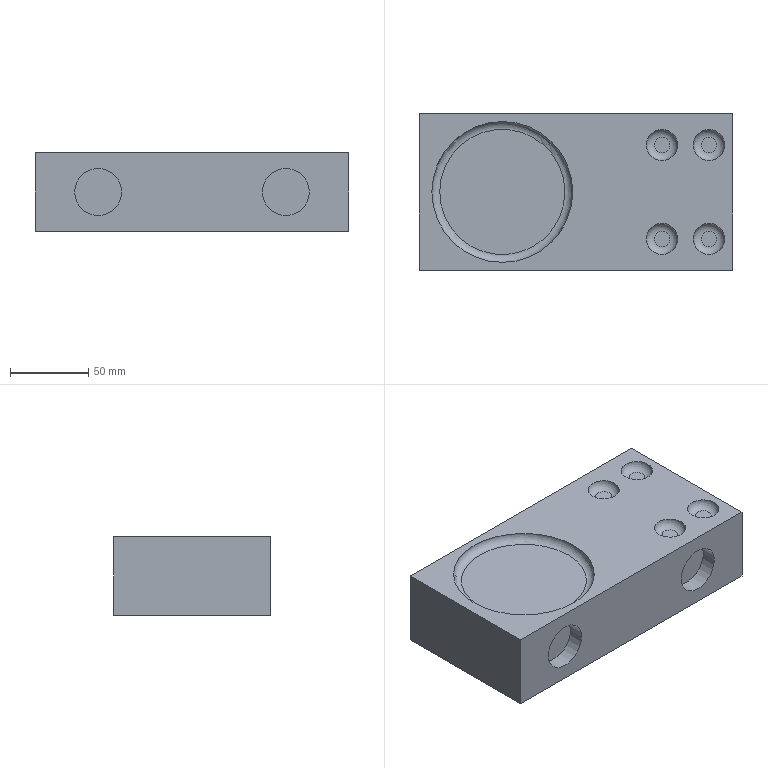Part | NX | features EXTRUDE 4, DATUM_CSYS 3, BLEND 2, SKETCH 2 | 1 solid | 20 faces | box 200 x 100 x 50 mm | volume 950448 mm3 | plane 13 | torus 5 | cylinder 2 | commonest cylinder face diameters 30 x2
STEP:
#1=CARTESIAN_POINT('',(75.,-50.,-25.));
#2=VERTEX_POINT('',#1);
#3=CARTESIAN_POINT('',(60.,-50.,-25.));
#4=DIRECTION('',(0.,-1.,0.));
#5=DIRECTION('',(1.,0.,0.));
#6=AXIS2_PLACEMENT_3D('',#3,#4,#5);
#7=CIRCLE('',#6,15.);
#8=EDGE_CURVE('',#2,#2,#7,.T.);
#9=ORIENTED_EDGE('',*,*,#8,.F.);
#10=EDGE_LOOP('',(#9));
#11=FACE_BOUND('',#10,.T.);
#12=CARTESIAN_POINT('',(-45.,-50.,-25.));
#13=VERTEX_POINT('',#12);
#14=CARTESIAN_POINT('',(-60.,-50.,-25.));
#15=DIRECTION('',(0.,-1.,0.));
#16=DIRECTION('',(1.,0.,0.));
#17=AXIS2_PLACEMENT_3D('',#14,#15,#16);
#18=CIRCLE('',#17,15.);
#19=EDGE_CURVE('',#13,#13,#18,.T.);
#20=ORIENTED_EDGE('',*,*,#19,.F.);
#21=EDGE_LOOP('',(#20));
#22=FACE_BOUND('',#21,.T.);
#23=CARTESIAN_POINT('',(100.,-50.,0.));
#24=VERTEX_POINT('',#23);
#25=CARTESIAN_POINT('',(-100.,-50.,0.));
#26=VERTEX_POINT('',#25);
#27=CARTESIAN_POINT('',(100.,-50.,0.));
#28=DIRECTION('',(-1.,0.,0.));
#29=VECTOR('',#28,1000.);
#30=LINE('',#27,#29);
#31=EDGE_CURVE('',#24,#26,#30,.T.);
#32=ORIENTED_EDGE('',*,*,#31,.T.);
#33=CARTESIAN_POINT('',(-100.,-50.,-50.));
#34=VERTEX_POINT('',#33);
#35=CARTESIAN_POINT('',(-100.,-50.,-50.));
#36=DIRECTION('',(0.,0.,1.));
#37=VECTOR('',#36,1000.);
#38=LINE('',#35,#37);
#39=EDGE_CURVE('',#34,#26,#38,.T.);
#40=ORIENTED_EDGE('',*,*,#39,.F.);
#41=CARTESIAN_POINT('',(100.,-50.,-50.));
#42=VERTEX_POINT('',#41);
#43=CARTESIAN_POINT('',(100.,-50.,-50.));
#44=DIRECTION('',(-1.,0.,0.));
#45=VECTOR('',#44,1000.);
#46=LINE('',#43,#45);
#47=EDGE_CURVE('',#42,#34,#46,.T.);
#48=ORIENTED_EDGE('',*,*,#47,.F.);
#49=CARTESIAN_POINT('',(100.,-50.,-50.));
#50=DIRECTION('',(0.,0.,1.));
#51=VECTOR('',#50,1000.);
#52=LINE('',#49,#51);
#53=EDGE_CURVE('',#42,#24,#52,.T.);
#54=ORIENTED_EDGE('',*,*,#53,.T.);
#55=EDGE_LOOP('',(#32,#40,#48,#54));
#56=FACE_BOUND('',#55,.T.);
#57=CARTESIAN_POINT('',(100.,-50.,-50.));
#58=DIRECTION('',(0.,1.,0.));
#59=DIRECTION('',(0.,0.,1.));
#60=AXIS2_PLACEMENT_3D('',#57,#58,#59);
#61=PLANE('',#60);
#62=ADVANCED_FACE('',(#11,#22,#56),#61,.F.);
#63=CARTESIAN_POINT('',(-100.,50.,0.));
#64=VERTEX_POINT('',#63);
#65=CARTESIAN_POINT('',(-100.,-50.,0.));
#66=DIRECTION('',(0.,1.,0.));
#67=VECTOR('',#66,1000.);
#68=LINE('',#65,#67);
#69=EDGE_CURVE('',#26,#64,#68,.T.);
#70=ORIENTED_EDGE('',*,*,#69,.T.);
#71=CARTESIAN_POINT('',(-100.,50.,-50.));
#72=VERTEX_POINT('',#71);
#73=CARTESIAN_POINT('',(-100.,50.,-50.));
#74=DIRECTION('',(0.,0.,1.));
#75=VECTOR('',#74,1000.);
#76=LINE('',#73,#75);
#77=EDGE_CURVE('',#72,#64,#76,.T.);
#78=ORIENTED_EDGE('',*,*,#77,.F.);
#79=CARTESIAN_POINT('',(-100.,-50.,-50.));
#80=DIRECTION('',(0.,1.,0.));
#81=VECTOR('',#80,1000.);
#82=LINE('',#79,#81);
#83=EDGE_CURVE('',#34,#72,#82,.T.);
#84=ORIENTED_EDGE('',*,*,#83,.F.);
#85=ORIENTED_EDGE('',*,*,#39,.T.);
#86=EDGE_LOOP('',(#70,#78,#84,#85));
#87=FACE_BOUND('',#86,.T.);
#88=CARTESIAN_POINT('',(-100.,-50.,-50.));
#89=DIRECTION('',(1.,0.,0.));
#90=DIRECTION('',(0.,0.,-1.));
#91=AXIS2_PLACEMENT_3D('',#88,#89,#90);
#92=PLANE('',#91);
#93=ADVANCED_FACE('',(#87),#92,.F.);
#94=CARTESIAN_POINT('',(100.,50.,0.));
#95=VERTEX_POINT('',#94);
#96=CARTESIAN_POINT('',(-100.,50.,0.));
#97=DIRECTION('',(1.,0.,0.));
#98=VECTOR('',#97,1000.);
#99=LINE('',#96,#98);
#100=EDGE_CURVE('',#64,#95,#99,.T.);
#101=ORIENTED_EDGE('',*,*,#100,.T.);
#102=CARTESIAN_POINT('',(100.,50.,-50.));
#103=VERTEX_POINT('',#102);
#104=CARTESIAN_POINT('',(100.,50.,-50.));
#105=DIRECTION('',(0.,0.,1.));
#106=VECTOR('',#105,1000.);
#107=LINE('',#104,#106);
#108=EDGE_CURVE('',#103,#95,#107,.T.);
#109=ORIENTED_EDGE('',*,*,#108,.F.);
#110=CARTESIAN_POINT('',(-100.,50.,-50.));
#111=DIRECTION('',(1.,0.,0.));
#112=VECTOR('',#111,1000.);
#113=LINE('',#110,#112);
#114=EDGE_CURVE('',#72,#103,#113,.T.);
#115=ORIENTED_EDGE('',*,*,#114,.F.);
#116=ORIENTED_EDGE('',*,*,#77,.T.);
#117=EDGE_LOOP('',(#101,#109,#115,#116));
#118=FACE_BOUND('',#117,.T.);
#119=CARTESIAN_POINT('',(-100.,50.,-50.));
#120=DIRECTION('',(0.,-1.,0.));
#121=DIRECTION('',(0.,0.,-1.));
#122=AXIS2_PLACEMENT_3D('',#119,#120,#121);
#123=PLANE('',#122);
#124=ADVANCED_FACE('',(#118),#123,.F.);
#125=CARTESIAN_POINT('',(100.,50.,0.));
#126=DIRECTION('',(0.,-1.,0.));
#127=VECTOR('',#126,1000.);
#128=LINE('',#125,#127);
#129=EDGE_CURVE('',#95,#24,#128,.T.);
#130=ORIENTED_EDGE('',*,*,#129,.T.);
#131=ORIENTED_EDGE('',*,*,#53,.F.);
#132=CARTESIAN_POINT('',(100.,50.,-50.));
#133=DIRECTION('',(0.,-1.,0.));
#134=VECTOR('',#133,1000.);
#135=LINE('',#132,#134);
#136=EDGE_CURVE('',#103,#42,#135,.T.);
#137=ORIENTED_EDGE('',*,*,#136,.F.);
#138=ORIENTED_EDGE('',*,*,#108,.T.);
#139=EDGE_LOOP('',(#130,#131,#137,#138));
#140=FACE_BOUND('',#139,.T.);
#141=CARTESIAN_POINT('',(100.,50.,-50.));
#142=DIRECTION('',(-1.,0.,0.));
#143=DIRECTION('',(0.,0.,1.));
#144=AXIS2_PLACEMENT_3D('',#141,#142,#143);
#145=PLANE('',#144);
#146=ADVANCED_FACE('',(#140),#145,.F.);
#147=ORIENTED_EDGE('',*,*,#47,.T.);
#148=ORIENTED_EDGE('',*,*,#83,.T.);
#149=ORIENTED_EDGE('',*,*,#114,.T.);
#150=ORIENTED_EDGE('',*,*,#136,.T.);
#151=EDGE_LOOP('',(#147,#148,#149,#150));
#152=FACE_BOUND('',#151,.T.);
#153=CARTESIAN_POINT('',(0.,0.,-50.));
#154=DIRECTION('',(0.,0.,-1.));
#155=DIRECTION('',(-1.,0.,0.));
#156=AXIS2_PLACEMENT_3D('',#153,#154,#155);
#157=PLANE('',#156);
#158=ADVANCED_FACE('',(#152),#157,.T.);
#159=CARTESIAN_POINT('',(95.,30.,0.));
#160=VERTEX_POINT('',#159);
#161=CARTESIAN_POINT('',(85.,30.,0.));
#162=DIRECTION('',(0.,0.,-1.));
#163=DIRECTION('',(1.,0.,0.));
#164=AXIS2_PLACEMENT_3D('',#161,#162,#163);
#165=CIRCLE('',#164,10.);
#166=EDGE_CURVE('',#160,#160,#165,.T.);
#167=ORIENTED_EDGE('',*,*,#166,.T.);
#168=EDGE_LOOP('',(#167));
#169=FACE_BOUND('',#168,.T.);
#170=CARTESIAN_POINT('',(65.,-30.,0.));
#171=VERTEX_POINT('',#170);
#172=CARTESIAN_POINT('',(55.,-30.,0.));
#173=DIRECTION('',(0.,0.,-1.));
#174=DIRECTION('',(1.,0.,0.));
#175=AXIS2_PLACEMENT_3D('',#172,#173,#174);
#176=CIRCLE('',#175,10.);
#177=EDGE_CURVE('',#171,#171,#176,.T.);
#178=ORIENTED_EDGE('',*,*,#177,.T.);
#179=EDGE_LOOP('',(#178));
#180=FACE_BOUND('',#179,.T.);
#181=CARTESIAN_POINT('',(65.,30.,0.));
#182=VERTEX_POINT('',#181);
#183=CARTESIAN_POINT('',(55.,30.,0.));
#184=DIRECTION('',(0.,0.,1.));
#185=DIRECTION('',(1.,0.,0.));
#186=AXIS2_PLACEMENT_3D('',#183,#184,#185);
#187=CIRCLE('',#186,10.);
#188=EDGE_CURVE('',#182,#182,#187,.T.);
#189=ORIENTED_EDGE('',*,*,#188,.F.);
#190=EDGE_LOOP('',(#189));
#191=FACE_BOUND('',#190,.T.);
#192=CARTESIAN_POINT('',(95.,-30.,0.));
#193=VERTEX_POINT('',#192);
#194=CARTESIAN_POINT('',(85.,-30.,0.));
#195=DIRECTION('',(0.,0.,-1.));
#196=DIRECTION('',(1.,0.,0.));
#197=AXIS2_PLACEMENT_3D('',#194,#195,#196);
#198=CIRCLE('',#197,10.);
#199=EDGE_CURVE('',#193,#193,#198,.T.);
#200=ORIENTED_EDGE('',*,*,#199,.T.);
#201=EDGE_LOOP('',(#200));
#202=FACE_BOUND('',#201,.T.);
#203=CARTESIAN_POINT('',(-2.088,0.,0.));
#204=VERTEX_POINT('',#203);
#205=CARTESIAN_POINT('',(-47.088,0.,0.));
#206=DIRECTION('',(0.,0.,1.));
#207=DIRECTION('',(1.,0.,0.));
#208=AXIS2_PLACEMENT_3D('',#205,#206,#207);
#209=CIRCLE('',#208,45.);
#210=EDGE_CURVE('',#204,#204,#209,.T.);
#211=ORIENTED_EDGE('',*,*,#210,.F.);
#212=EDGE_LOOP('',(#211));
#213=FACE_BOUND('',#212,.T.);
#214=ORIENTED_EDGE('',*,*,#31,.F.);
#215=ORIENTED_EDGE('',*,*,#129,.F.);
#216=ORIENTED_EDGE('',*,*,#100,.F.);
#217=ORIENTED_EDGE('',*,*,#69,.F.);
#218=EDGE_LOOP('',(#214,#215,#216,#217));
#219=FACE_BOUND('',#218,.T.);
#220=CARTESIAN_POINT('',(0.,0.,0.));
#221=DIRECTION('',(0.,0.,-1.));
#222=DIRECTION('',(-1.,0.,0.));
#223=AXIS2_PLACEMENT_3D('',#220,#221,#222);
#224=PLANE('',#223);
#225=ADVANCED_FACE('',(#169,#180,#191,#202,#213,#219),#224,.F.);
#226=CARTESIAN_POINT('',(-7.088,0.,-5.));
#227=VERTEX_POINT('',#226);
#228=CARTESIAN_POINT('',(-47.088,0.,-5.));
#229=DIRECTION('',(0.,0.,1.));
#230=DIRECTION('',(1.,0.,0.));
#231=AXIS2_PLACEMENT_3D('',#228,#229,#230);
#232=CIRCLE('',#231,40.);
#233=EDGE_CURVE('',#227,#227,#232,.T.);
#234=ORIENTED_EDGE('',*,*,#233,.T.);
#235=EDGE_LOOP('',(#234));
#236=FACE_BOUND('',#235,.T.);
#237=CARTESIAN_POINT('',(-47.088,0.,-5.));
#238=DIRECTION('',(0.,0.,1.));
#239=DIRECTION('',(1.,0.,0.));
#240=AXIS2_PLACEMENT_3D('',#237,#238,#239);
#241=PLANE('',#240);
#242=ADVANCED_FACE('',(#236),#241,.T.);
#243=CARTESIAN_POINT('',(80.,-30.,-5.));
#244=VERTEX_POINT('',#243);
#245=CARTESIAN_POINT('',(85.,-30.,-5.));
#246=DIRECTION('',(0.,0.,-1.));
#247=DIRECTION('',(-1.,0.,0.));
#248=AXIS2_PLACEMENT_3D('',#245,#246,#247);
#249=CIRCLE('',#248,5.);
#250=EDGE_CURVE('',#244,#244,#249,.F.);
#251=ORIENTED_EDGE('',*,*,#250,.T.);
#252=EDGE_LOOP('',(#251));
#253=FACE_BOUND('',#252,.T.);
#254=CARTESIAN_POINT('',(85.,-30.,-5.));
#255=DIRECTION('',(0.,0.,-1.));
#256=DIRECTION('',(-1.,0.,0.));
#257=AXIS2_PLACEMENT_3D('',#254,#255,#256);
#258=PLANE('',#257);
#259=ADVANCED_FACE('',(#253),#258,.F.);
#260=CARTESIAN_POINT('',(60.,30.,-5.));
#261=VERTEX_POINT('',#260);
#262=CARTESIAN_POINT('',(55.,30.,-5.));
#263=DIRECTION('',(0.,0.,1.));
#264=DIRECTION('',(1.,0.,0.));
#265=AXIS2_PLACEMENT_3D('',#262,#263,#264);
#266=CIRCLE('',#265,5.);
#267=EDGE_CURVE('',#261,#261,#266,.T.);
#268=ORIENTED_EDGE('',*,*,#267,.T.);
#269=EDGE_LOOP('',(#268));
#270=FACE_BOUND('',#269,.T.);
#271=CARTESIAN_POINT('',(55.,30.,-5.));
#272=DIRECTION('',(0.,0.,1.));
#273=DIRECTION('',(1.,0.,0.));
#274=AXIS2_PLACEMENT_3D('',#271,#272,#273);
#275=PLANE('',#274);
#276=ADVANCED_FACE('',(#270),#275,.T.);
#277=CARTESIAN_POINT('',(50.,-30.,-5.));
#278=VERTEX_POINT('',#277);
#279=CARTESIAN_POINT('',(55.,-30.,-5.));
#280=DIRECTION('',(0.,0.,-1.));
#281=DIRECTION('',(-1.,0.,0.));
#282=AXIS2_PLACEMENT_3D('',#279,#280,#281);
#283=CIRCLE('',#282,5.);
#284=EDGE_CURVE('',#278,#278,#283,.F.);
#285=ORIENTED_EDGE('',*,*,#284,.T.);
#286=EDGE_LOOP('',(#285));
#287=FACE_BOUND('',#286,.T.);
#288=CARTESIAN_POINT('',(55.,-30.,-5.));
#289=DIRECTION('',(0.,0.,-1.));
#290=DIRECTION('',(-1.,0.,0.));
#291=AXIS2_PLACEMENT_3D('',#288,#289,#290);
#292=PLANE('',#291);
#293=ADVANCED_FACE('',(#287),#292,.F.);
#294=CARTESIAN_POINT('',(80.,30.,-5.));
#295=VERTEX_POINT('',#294);
#296=CARTESIAN_POINT('',(85.,30.,-5.));
#297=DIRECTION('',(0.,0.,-1.));
#298=DIRECTION('',(-1.,0.,0.));
#299=AXIS2_PLACEMENT_3D('',#296,#297,#298);
#300=CIRCLE('',#299,5.);
#301=EDGE_CURVE('',#295,#295,#300,.F.);
#302=ORIENTED_EDGE('',*,*,#301,.T.);
#303=EDGE_LOOP('',(#302));
#304=FACE_BOUND('',#303,.T.);
#305=CARTESIAN_POINT('',(85.,30.,-5.));
#306=DIRECTION('',(0.,0.,-1.));
#307=DIRECTION('',(-1.,0.,0.));
#308=AXIS2_PLACEMENT_3D('',#305,#306,#307);
#309=PLANE('',#308);
#310=ADVANCED_FACE('',(#304),#309,.F.);
#311=ORIENTED_EDGE('',*,*,#233,.F.);
#312=EDGE_LOOP('',(#311));
#313=FACE_BOUND('',#312,.T.);
#314=ORIENTED_EDGE('',*,*,#210,.T.);
#315=EDGE_LOOP('',(#314));
#316=FACE_BOUND('',#315,.T.);
#317=CARTESIAN_POINT('',(-47.088,0.,0.));
#318=DIRECTION('',(0.,0.,1.));
#319=DIRECTION('',(1.,0.,0.));
#320=AXIS2_PLACEMENT_3D('',#317,#318,#319);
#321=TOROIDAL_SURFACE('',#320,40.,5.);
#322=ADVANCED_FACE('',(#313,#316),#321,.F.);
#323=ORIENTED_EDGE('',*,*,#199,.F.);
#324=EDGE_LOOP('',(#323));
#325=FACE_BOUND('',#324,.T.);
#326=ORIENTED_EDGE('',*,*,#250,.F.);
#327=EDGE_LOOP('',(#326));
#328=FACE_BOUND('',#327,.T.);
#329=CARTESIAN_POINT('',(85.,-30.,0.));
#330=DIRECTION('',(0.,0.,-1.));
#331=DIRECTION('',(-1.,0.,0.));
#332=AXIS2_PLACEMENT_3D('',#329,#330,#331);
#333=TOROIDAL_SURFACE('',#332,5.,5.);
#334=ADVANCED_FACE('',(#325,#328),#333,.F.);
#335=ORIENTED_EDGE('',*,*,#177,.F.);
#336=EDGE_LOOP('',(#335));
#337=FACE_BOUND('',#336,.T.);
#338=ORIENTED_EDGE('',*,*,#284,.F.);
#339=EDGE_LOOP('',(#338));
#340=FACE_BOUND('',#339,.T.);
#341=CARTESIAN_POINT('',(55.,-30.,0.));
#342=DIRECTION('',(0.,0.,-1.));
#343=DIRECTION('',(-1.,0.,0.));
#344=AXIS2_PLACEMENT_3D('',#341,#342,#343);
#345=TOROIDAL_SURFACE('',#344,5.,5.);
#346=ADVANCED_FACE('',(#337,#340),#345,.F.);
#347=ORIENTED_EDGE('',*,*,#166,.F.);
#348=EDGE_LOOP('',(#347));
#349=FACE_BOUND('',#348,.T.);
#350=ORIENTED_EDGE('',*,*,#301,.F.);
#351=EDGE_LOOP('',(#350));
#352=FACE_BOUND('',#351,.T.);
#353=CARTESIAN_POINT('',(85.,30.,0.));
#354=DIRECTION('',(0.,0.,-1.));
#355=DIRECTION('',(-1.,0.,0.));
#356=AXIS2_PLACEMENT_3D('',#353,#354,#355);
#357=TOROIDAL_SURFACE('',#356,5.,5.);
#358=ADVANCED_FACE('',(#349,#352),#357,.F.);
#359=ORIENTED_EDGE('',*,*,#267,.F.);
#360=EDGE_LOOP('',(#359));
#361=FACE_BOUND('',#360,.T.);
#362=ORIENTED_EDGE('',*,*,#188,.T.);
#363=EDGE_LOOP('',(#362));
#364=FACE_BOUND('',#363,.T.);
#365=CARTESIAN_POINT('',(55.,30.,0.));
#366=DIRECTION('',(0.,0.,1.));
#367=DIRECTION('',(1.,0.,0.));
#368=AXIS2_PLACEMENT_3D('',#365,#366,#367);
#369=TOROIDAL_SURFACE('',#368,5.,5.);
#370=ADVANCED_FACE('',(#361,#364),#369,.F.);
#371=CARTESIAN_POINT('',(-45.,-40.,-25.));
#372=VERTEX_POINT('',#371);
#373=CARTESIAN_POINT('',(-60.,-40.,-25.));
#374=DIRECTION('',(0.,-1.,0.));
#375=DIRECTION('',(1.,0.,0.));
#376=AXIS2_PLACEMENT_3D('',#373,#374,#375);
#377=CIRCLE('',#376,15.);
#378=EDGE_CURVE('',#372,#372,#377,.F.);
#379=ORIENTED_EDGE('',*,*,#378,.T.);
#380=EDGE_LOOP('',(#379));
#381=FACE_BOUND('',#380,.T.);
#382=ORIENTED_EDGE('',*,*,#19,.T.);
#383=EDGE_LOOP('',(#382));
#384=FACE_BOUND('',#383,.T.);
#385=CARTESIAN_POINT('',(-60.,-40.,-25.));
#386=DIRECTION('',(0.,-1.,0.));
#387=DIRECTION('',(0.,0.,-1.));
#388=AXIS2_PLACEMENT_3D('',#385,#386,#387);
#389=CYLINDRICAL_SURFACE('',#388,15.);
#390=ADVANCED_FACE('',(#381,#384),#389,.F.);
#391=ORIENTED_EDGE('',*,*,#378,.F.);
#392=EDGE_LOOP('',(#391));
#393=FACE_BOUND('',#392,.T.);
#394=CARTESIAN_POINT('',(-60.,-40.,-25.));
#395=DIRECTION('',(0.,-1.,0.));
#396=DIRECTION('',(0.,0.,-1.));
#397=AXIS2_PLACEMENT_3D('',#394,#395,#396);
#398=PLANE('',#397);
#399=ADVANCED_FACE('',(#393),#398,.T.);
#400=CARTESIAN_POINT('',(75.,-40.,-25.));
#401=VERTEX_POINT('',#400);
#402=CARTESIAN_POINT('',(60.,-40.,-25.));
#403=DIRECTION('',(0.,-1.,0.));
#404=DIRECTION('',(1.,0.,0.));
#405=AXIS2_PLACEMENT_3D('',#402,#403,#404);
#406=CIRCLE('',#405,15.);
#407=EDGE_CURVE('',#401,#401,#406,.F.);
#408=ORIENTED_EDGE('',*,*,#407,.T.);
#409=EDGE_LOOP('',(#408));
#410=FACE_BOUND('',#409,.T.);
#411=ORIENTED_EDGE('',*,*,#8,.T.);
#412=EDGE_LOOP('',(#411));
#413=FACE_BOUND('',#412,.T.);
#414=CARTESIAN_POINT('',(60.,-40.,-25.));
#415=DIRECTION('',(0.,-1.,0.));
#416=DIRECTION('',(0.,0.,-1.));
#417=AXIS2_PLACEMENT_3D('',#414,#415,#416);
#418=CYLINDRICAL_SURFACE('',#417,15.);
#419=ADVANCED_FACE('',(#410,#413),#418,.F.);
#420=ORIENTED_EDGE('',*,*,#407,.F.);
#421=EDGE_LOOP('',(#420));
#422=FACE_BOUND('',#421,.T.);
#423=CARTESIAN_POINT('',(60.,-40.,-25.));
#424=DIRECTION('',(0.,-1.,0.));
#425=DIRECTION('',(0.,0.,-1.));
#426=AXIS2_PLACEMENT_3D('',#423,#424,#425);
#427=PLANE('',#426);
#428=ADVANCED_FACE('',(#422),#427,.T.);
#429=CLOSED_SHELL('',(#62,#93,#124,#146,#158,#225,#242,#259,#276,#293,#310,#322,#334,#346,#358,#370,#390,#399,#419,#428));
#430=MANIFOLD_SOLID_BREP('',#429);
#431=(LENGTH_UNIT()NAMED_UNIT(*)SI_UNIT(.MILLI.,.METRE.));
#432=UNCERTAINTY_MEASURE_WITH_UNIT(LENGTH_MEASURE(0.00001),#431,'','');
#433=(NAMED_UNIT(*)PLANE_ANGLE_UNIT()SI_UNIT($,.RADIAN.));
#434=(NAMED_UNIT(*)SI_UNIT($,.STERADIAN.)SOLID_ANGLE_UNIT());
#435=(GEOMETRIC_REPRESENTATION_CONTEXT(3)GLOBAL_UNCERTAINTY_ASSIGNED_CONTEXT((#432))GLOBAL_UNIT_ASSIGNED_CONTEXT((#431,#433,#434))REPRESENTATION_CONTEXT('',''));
#436=ADVANCED_BREP_SHAPE_REPRESENTATION('',(#430),#435);